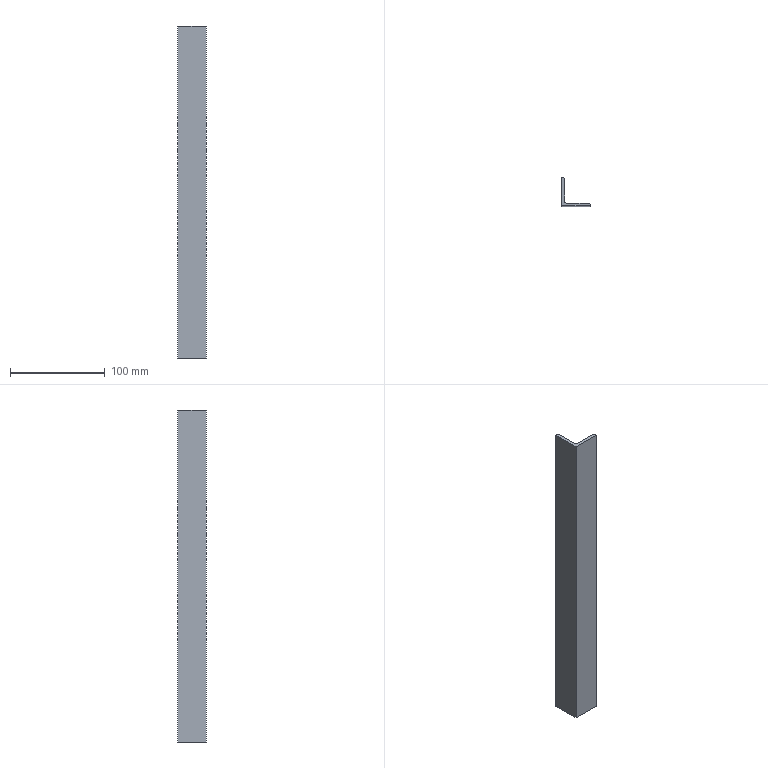Part | SolidWorks | features Extrusion 1 | 1 solid | 11 faces | box 30 x 30 x 350 mm | volume 59550 mm3 | plane 8 | cylinder 3 | commonest cylinder face diameters 4 x3
STEP:
#1=CARTESIAN_POINT('',(0.,30.,0.));
#2=VERTEX_POINT('',#1);
#3=CARTESIAN_POINT('',(0.,0.,0.));
#4=VERTEX_POINT('',#3);
#5=CARTESIAN_POINT('',(0.,0.,0.));
#6=DIRECTION('',(0.,-1.,0.));
#7=VECTOR('',#6,1000.);
#8=LINE('',#5,#7);
#9=EDGE_CURVE('',#2,#4,#8,.T.);
#10=ORIENTED_EDGE('',*,*,#9,.T.);
#11=CARTESIAN_POINT('',(0.,0.,350.));
#12=VERTEX_POINT('',#11);
#13=CARTESIAN_POINT('',(0.,0.,350.));
#14=DIRECTION('',(0.,0.,-1.));
#15=VECTOR('',#14,1000.);
#16=LINE('',#13,#15);
#17=EDGE_CURVE('',#12,#4,#16,.T.);
#18=ORIENTED_EDGE('',*,*,#17,.F.);
#19=CARTESIAN_POINT('',(0.,30.,350.));
#20=VERTEX_POINT('',#19);
#21=CARTESIAN_POINT('',(0.,0.,350.));
#22=DIRECTION('',(0.,-1.,0.));
#23=VECTOR('',#22,1000.);
#24=LINE('',#21,#23);
#25=EDGE_CURVE('',#20,#12,#24,.T.);
#26=ORIENTED_EDGE('',*,*,#25,.F.);
#27=CARTESIAN_POINT('',(0.,30.,350.));
#28=DIRECTION('',(0.,0.,-1.));
#29=VECTOR('',#28,1000.);
#30=LINE('',#27,#29);
#31=EDGE_CURVE('',#20,#2,#30,.T.);
#32=ORIENTED_EDGE('',*,*,#31,.T.);
#33=EDGE_LOOP('',(#10,#18,#26,#32));
#34=FACE_OUTER_BOUND('',#33,.T.);
#35=CARTESIAN_POINT('',(0.,0.,350.));
#36=DIRECTION('',(1.,0.,0.));
#37=DIRECTION('',(0.,0.,-1.));
#38=AXIS2_PLACEMENT_3D('',#35,#36,#37);
#39=PLANE('',#38);
#40=ADVANCED_FACE('',(#34),#39,.F.);
#41=CARTESIAN_POINT('',(30.,0.,0.));
#42=VERTEX_POINT('',#41);
#43=CARTESIAN_POINT('',(0.,0.,0.));
#44=DIRECTION('',(1.,0.,0.));
#45=VECTOR('',#44,1000.);
#46=LINE('',#43,#45);
#47=EDGE_CURVE('',#4,#42,#46,.T.);
#48=ORIENTED_EDGE('',*,*,#47,.T.);
#49=CARTESIAN_POINT('',(30.,0.,350.));
#50=VERTEX_POINT('',#49);
#51=CARTESIAN_POINT('',(30.,0.,350.));
#52=DIRECTION('',(0.,0.,-1.));
#53=VECTOR('',#52,1000.);
#54=LINE('',#51,#53);
#55=EDGE_CURVE('',#50,#42,#54,.T.);
#56=ORIENTED_EDGE('',*,*,#55,.F.);
#57=CARTESIAN_POINT('',(0.,0.,350.));
#58=DIRECTION('',(1.,0.,0.));
#59=VECTOR('',#58,1000.);
#60=LINE('',#57,#59);
#61=EDGE_CURVE('',#12,#50,#60,.T.);
#62=ORIENTED_EDGE('',*,*,#61,.F.);
#63=ORIENTED_EDGE('',*,*,#17,.T.);
#64=EDGE_LOOP('',(#48,#56,#62,#63));
#65=FACE_OUTER_BOUND('',#64,.T.);
#66=CARTESIAN_POINT('',(0.,0.,350.));
#67=DIRECTION('',(0.,1.,0.));
#68=DIRECTION('',(0.,0.,1.));
#69=AXIS2_PLACEMENT_3D('',#66,#67,#68);
#70=PLANE('',#69);
#71=ADVANCED_FACE('',(#65),#70,.F.);
#72=CARTESIAN_POINT('',(30.,1.,0.));
#73=VERTEX_POINT('',#72);
#74=CARTESIAN_POINT('',(30.,1.,0.));
#75=DIRECTION('',(0.,1.,0.));
#76=VECTOR('',#75,1000.);
#77=LINE('',#74,#76);
#78=EDGE_CURVE('',#42,#73,#77,.T.);
#79=ORIENTED_EDGE('',*,*,#78,.T.);
#80=CARTESIAN_POINT('',(30.,1.,350.));
#81=VERTEX_POINT('',#80);
#82=CARTESIAN_POINT('',(30.,1.,350.));
#83=DIRECTION('',(0.,0.,-1.));
#84=VECTOR('',#83,1000.);
#85=LINE('',#82,#84);
#86=EDGE_CURVE('',#81,#73,#85,.T.);
#87=ORIENTED_EDGE('',*,*,#86,.F.);
#88=CARTESIAN_POINT('',(30.,1.,350.));
#89=DIRECTION('',(0.,1.,0.));
#90=VECTOR('',#89,1000.);
#91=LINE('',#88,#90);
#92=EDGE_CURVE('',#50,#81,#91,.T.);
#93=ORIENTED_EDGE('',*,*,#92,.F.);
#94=ORIENTED_EDGE('',*,*,#55,.T.);
#95=EDGE_LOOP('',(#79,#87,#93,#94));
#96=FACE_OUTER_BOUND('',#95,.T.);
#97=CARTESIAN_POINT('',(30.,1.,350.));
#98=DIRECTION('',(-1.,0.,0.));
#99=DIRECTION('',(0.,0.,1.));
#100=AXIS2_PLACEMENT_3D('',#97,#98,#99);
#101=PLANE('',#100);
#102=ADVANCED_FACE('',(#96),#101,.F.);
#103=CARTESIAN_POINT('',(28.,3.,0.));
#104=VERTEX_POINT('',#103);
#105=CARTESIAN_POINT('',(28.,1.,0.));
#106=DIRECTION('',(0.,0.,1.));
#107=DIRECTION('',(1.,0.,0.));
#108=AXIS2_PLACEMENT_3D('',#105,#106,#107);
#109=CIRCLE('',#108,2.);
#110=EDGE_CURVE('',#73,#104,#109,.T.);
#111=ORIENTED_EDGE('',*,*,#110,.T.);
#112=CARTESIAN_POINT('',(28.,3.,350.));
#113=VERTEX_POINT('',#112);
#114=CARTESIAN_POINT('',(28.,3.,350.));
#115=DIRECTION('',(0.,0.,-1.));
#116=VECTOR('',#115,1000.);
#117=LINE('',#114,#116);
#118=EDGE_CURVE('',#113,#104,#117,.T.);
#119=ORIENTED_EDGE('',*,*,#118,.F.);
#120=CARTESIAN_POINT('',(28.,1.,350.));
#121=DIRECTION('',(0.,0.,1.));
#122=DIRECTION('',(1.,0.,0.));
#123=AXIS2_PLACEMENT_3D('',#120,#121,#122);
#124=CIRCLE('',#123,2.);
#125=EDGE_CURVE('',#81,#113,#124,.T.);
#126=ORIENTED_EDGE('',*,*,#125,.F.);
#127=ORIENTED_EDGE('',*,*,#86,.T.);
#128=EDGE_LOOP('',(#111,#119,#126,#127));
#129=FACE_OUTER_BOUND('',#128,.T.);
#130=CARTESIAN_POINT('',(28.,1.,350.));
#131=DIRECTION('',(0.,0.,-1.));
#132=DIRECTION('',(-1.,0.,0.));
#133=AXIS2_PLACEMENT_3D('',#130,#131,#132);
#134=CYLINDRICAL_SURFACE('',#133,2.);
#135=ADVANCED_FACE('',(#129),#134,.T.);
#136=CARTESIAN_POINT('',(5.,3.,0.));
#137=VERTEX_POINT('',#136);
#138=CARTESIAN_POINT('',(5.,3.,0.));
#139=DIRECTION('',(-1.,0.,0.));
#140=VECTOR('',#139,1000.);
#141=LINE('',#138,#140);
#142=EDGE_CURVE('',#104,#137,#141,.T.);
#143=ORIENTED_EDGE('',*,*,#142,.T.);
#144=CARTESIAN_POINT('',(5.,3.,350.));
#145=VERTEX_POINT('',#144);
#146=CARTESIAN_POINT('',(5.,3.,350.));
#147=DIRECTION('',(0.,0.,-1.));
#148=VECTOR('',#147,1000.);
#149=LINE('',#146,#148);
#150=EDGE_CURVE('',#145,#137,#149,.T.);
#151=ORIENTED_EDGE('',*,*,#150,.F.);
#152=CARTESIAN_POINT('',(5.,3.,350.));
#153=DIRECTION('',(-1.,0.,0.));
#154=VECTOR('',#153,1000.);
#155=LINE('',#152,#154);
#156=EDGE_CURVE('',#113,#145,#155,.T.);
#157=ORIENTED_EDGE('',*,*,#156,.F.);
#158=ORIENTED_EDGE('',*,*,#118,.T.);
#159=EDGE_LOOP('',(#143,#151,#157,#158));
#160=FACE_OUTER_BOUND('',#159,.T.);
#161=CARTESIAN_POINT('',(5.,3.,350.));
#162=DIRECTION('',(0.,-1.,0.));
#163=DIRECTION('',(0.,0.,-1.));
#164=AXIS2_PLACEMENT_3D('',#161,#162,#163);
#165=PLANE('',#164);
#166=ADVANCED_FACE('',(#160),#165,.F.);
#167=CARTESIAN_POINT('',(3.,5.,0.));
#168=VERTEX_POINT('',#167);
#169=CARTESIAN_POINT('',(5.,5.,0.));
#170=DIRECTION('',(0.,0.,-1.));
#171=DIRECTION('',(-1.,0.,0.));
#172=AXIS2_PLACEMENT_3D('',#169,#170,#171);
#173=CIRCLE('',#172,2.);
#174=EDGE_CURVE('',#137,#168,#173,.T.);
#175=ORIENTED_EDGE('',*,*,#174,.T.);
#176=CARTESIAN_POINT('',(3.,5.,350.));
#177=VERTEX_POINT('',#176);
#178=CARTESIAN_POINT('',(3.,5.,350.));
#179=DIRECTION('',(0.,0.,-1.));
#180=VECTOR('',#179,1000.);
#181=LINE('',#178,#180);
#182=EDGE_CURVE('',#177,#168,#181,.T.);
#183=ORIENTED_EDGE('',*,*,#182,.F.);
#184=CARTESIAN_POINT('',(5.,5.,350.));
#185=DIRECTION('',(0.,0.,-1.));
#186=DIRECTION('',(-1.,0.,0.));
#187=AXIS2_PLACEMENT_3D('',#184,#185,#186);
#188=CIRCLE('',#187,2.);
#189=EDGE_CURVE('',#145,#177,#188,.T.);
#190=ORIENTED_EDGE('',*,*,#189,.F.);
#191=ORIENTED_EDGE('',*,*,#150,.T.);
#192=EDGE_LOOP('',(#175,#183,#190,#191));
#193=FACE_OUTER_BOUND('',#192,.T.);
#194=CARTESIAN_POINT('',(5.,5.,350.));
#195=DIRECTION('',(0.,0.,-1.));
#196=DIRECTION('',(-1.,0.,0.));
#197=AXIS2_PLACEMENT_3D('',#194,#195,#196);
#198=CYLINDRICAL_SURFACE('',#197,2.);
#199=ADVANCED_FACE('',(#193),#198,.F.);
#200=CARTESIAN_POINT('',(3.,28.,0.));
#201=VERTEX_POINT('',#200);
#202=CARTESIAN_POINT('',(3.,5.,0.));
#203=DIRECTION('',(0.,1.,0.));
#204=VECTOR('',#203,1000.);
#205=LINE('',#202,#204);
#206=EDGE_CURVE('',#168,#201,#205,.T.);
#207=ORIENTED_EDGE('',*,*,#206,.T.);
#208=CARTESIAN_POINT('',(3.,28.,350.));
#209=VERTEX_POINT('',#208);
#210=CARTESIAN_POINT('',(3.,28.,350.));
#211=DIRECTION('',(0.,0.,-1.));
#212=VECTOR('',#211,1000.);
#213=LINE('',#210,#212);
#214=EDGE_CURVE('',#209,#201,#213,.T.);
#215=ORIENTED_EDGE('',*,*,#214,.F.);
#216=CARTESIAN_POINT('',(3.,5.,350.));
#217=DIRECTION('',(0.,1.,0.));
#218=VECTOR('',#217,1000.);
#219=LINE('',#216,#218);
#220=EDGE_CURVE('',#177,#209,#219,.T.);
#221=ORIENTED_EDGE('',*,*,#220,.F.);
#222=ORIENTED_EDGE('',*,*,#182,.T.);
#223=EDGE_LOOP('',(#207,#215,#221,#222));
#224=FACE_OUTER_BOUND('',#223,.T.);
#225=CARTESIAN_POINT('',(3.,5.,350.));
#226=DIRECTION('',(-1.,0.,0.));
#227=DIRECTION('',(0.,0.,1.));
#228=AXIS2_PLACEMENT_3D('',#225,#226,#227);
#229=PLANE('',#228);
#230=ADVANCED_FACE('',(#224),#229,.F.);
#231=CARTESIAN_POINT('',(1.,30.,0.));
#232=VERTEX_POINT('',#231);
#233=CARTESIAN_POINT('',(1.,28.,0.));
#234=DIRECTION('',(0.,0.,1.));
#235=DIRECTION('',(1.,0.,0.));
#236=AXIS2_PLACEMENT_3D('',#233,#234,#235);
#237=CIRCLE('',#236,2.);
#238=EDGE_CURVE('',#201,#232,#237,.T.);
#239=ORIENTED_EDGE('',*,*,#238,.T.);
#240=CARTESIAN_POINT('',(1.,30.,350.));
#241=VERTEX_POINT('',#240);
#242=CARTESIAN_POINT('',(1.,30.,350.));
#243=DIRECTION('',(0.,0.,-1.));
#244=VECTOR('',#243,1000.);
#245=LINE('',#242,#244);
#246=EDGE_CURVE('',#241,#232,#245,.T.);
#247=ORIENTED_EDGE('',*,*,#246,.F.);
#248=CARTESIAN_POINT('',(1.,28.,350.));
#249=DIRECTION('',(0.,0.,1.));
#250=DIRECTION('',(1.,0.,0.));
#251=AXIS2_PLACEMENT_3D('',#248,#249,#250);
#252=CIRCLE('',#251,2.);
#253=EDGE_CURVE('',#209,#241,#252,.T.);
#254=ORIENTED_EDGE('',*,*,#253,.F.);
#255=ORIENTED_EDGE('',*,*,#214,.T.);
#256=EDGE_LOOP('',(#239,#247,#254,#255));
#257=FACE_OUTER_BOUND('',#256,.T.);
#258=CARTESIAN_POINT('',(1.,28.,350.));
#259=DIRECTION('',(0.,0.,-1.));
#260=DIRECTION('',(-1.,0.,0.));
#261=AXIS2_PLACEMENT_3D('',#258,#259,#260);
#262=CYLINDRICAL_SURFACE('',#261,2.);
#263=ADVANCED_FACE('',(#257),#262,.T.);
#264=CARTESIAN_POINT('',(0.,30.,0.));
#265=DIRECTION('',(-1.,0.,0.));
#266=VECTOR('',#265,1000.);
#267=LINE('',#264,#266);
#268=EDGE_CURVE('',#232,#2,#267,.T.);
#269=ORIENTED_EDGE('',*,*,#268,.T.);
#270=ORIENTED_EDGE('',*,*,#31,.F.);
#271=CARTESIAN_POINT('',(0.,30.,350.));
#272=DIRECTION('',(-1.,0.,0.));
#273=VECTOR('',#272,1000.);
#274=LINE('',#271,#273);
#275=EDGE_CURVE('',#241,#20,#274,.T.);
#276=ORIENTED_EDGE('',*,*,#275,.F.);
#277=ORIENTED_EDGE('',*,*,#246,.T.);
#278=EDGE_LOOP('',(#269,#270,#276,#277));
#279=FACE_OUTER_BOUND('',#278,.T.);
#280=CARTESIAN_POINT('',(0.,30.,350.));
#281=DIRECTION('',(0.,-1.,0.));
#282=DIRECTION('',(0.,0.,-1.));
#283=AXIS2_PLACEMENT_3D('',#280,#281,#282);
#284=PLANE('',#283);
#285=ADVANCED_FACE('',(#279),#284,.F.);
#286=ORIENTED_EDGE('',*,*,#25,.T.);
#287=ORIENTED_EDGE('',*,*,#61,.T.);
#288=ORIENTED_EDGE('',*,*,#92,.T.);
#289=ORIENTED_EDGE('',*,*,#125,.T.);
#290=ORIENTED_EDGE('',*,*,#156,.T.);
#291=ORIENTED_EDGE('',*,*,#189,.T.);
#292=ORIENTED_EDGE('',*,*,#220,.T.);
#293=ORIENTED_EDGE('',*,*,#253,.T.);
#294=ORIENTED_EDGE('',*,*,#275,.T.);
#295=EDGE_LOOP('',(#286,#287,#288,#289,#290,#291,#292,#293,#294));
#296=FACE_OUTER_BOUND('',#295,.T.);
#297=CARTESIAN_POINT('',(1.,28.,350.));
#298=DIRECTION('',(0.,0.,1.));
#299=DIRECTION('',(1.,0.,0.));
#300=AXIS2_PLACEMENT_3D('',#297,#298,#299);
#301=PLANE('',#300);
#302=ADVANCED_FACE('',(#296),#301,.T.);
#303=ORIENTED_EDGE('',*,*,#9,.F.);
#304=ORIENTED_EDGE('',*,*,#268,.F.);
#305=ORIENTED_EDGE('',*,*,#238,.F.);
#306=ORIENTED_EDGE('',*,*,#206,.F.);
#307=ORIENTED_EDGE('',*,*,#174,.F.);
#308=ORIENTED_EDGE('',*,*,#142,.F.);
#309=ORIENTED_EDGE('',*,*,#110,.F.);
#310=ORIENTED_EDGE('',*,*,#78,.F.);
#311=ORIENTED_EDGE('',*,*,#47,.F.);
#312=EDGE_LOOP('',(#303,#304,#305,#306,#307,#308,#309,#310,#311));
#313=FACE_OUTER_BOUND('',#312,.T.);
#314=CARTESIAN_POINT('',(1.,28.,0.));
#315=DIRECTION('',(0.,0.,1.));
#316=DIRECTION('',(1.,0.,0.));
#317=AXIS2_PLACEMENT_3D('',#314,#315,#316);
#318=PLANE('',#317);
#319=ADVANCED_FACE('',(#313),#318,.F.);
#320=CLOSED_SHELL('',(#40,#71,#102,#135,#166,#199,#230,#263,#285,#302,#319));
#321=MANIFOLD_SOLID_BREP('',#320);
#322=CARTESIAN_POINT('',(0.,0.,0.));
#323=DIRECTION('',(0.,0.,1.));
#324=DIRECTION('',(1.,0.,0.));
#325=AXIS2_PLACEMENT_3D('',#322,#323,#324);
#326=(LENGTH_UNIT()NAMED_UNIT(*)SI_UNIT(.MILLI.,.METRE.));
#327=UNCERTAINTY_MEASURE_WITH_UNIT(LENGTH_MEASURE(0.00001),#326,'','');
#328=(NAMED_UNIT(*)PLANE_ANGLE_UNIT()SI_UNIT($,.RADIAN.));
#329=(NAMED_UNIT(*)SI_UNIT($,.STERADIAN.)SOLID_ANGLE_UNIT());
#330=(GEOMETRIC_REPRESENTATION_CONTEXT(3)GLOBAL_UNCERTAINTY_ASSIGNED_CONTEXT((#327))GLOBAL_UNIT_ASSIGNED_CONTEXT((#326,#328,#329))REPRESENTATION_CONTEXT('',''));
#331=ADVANCED_BREP_SHAPE_REPRESENTATION('',(#321,#325),#330);